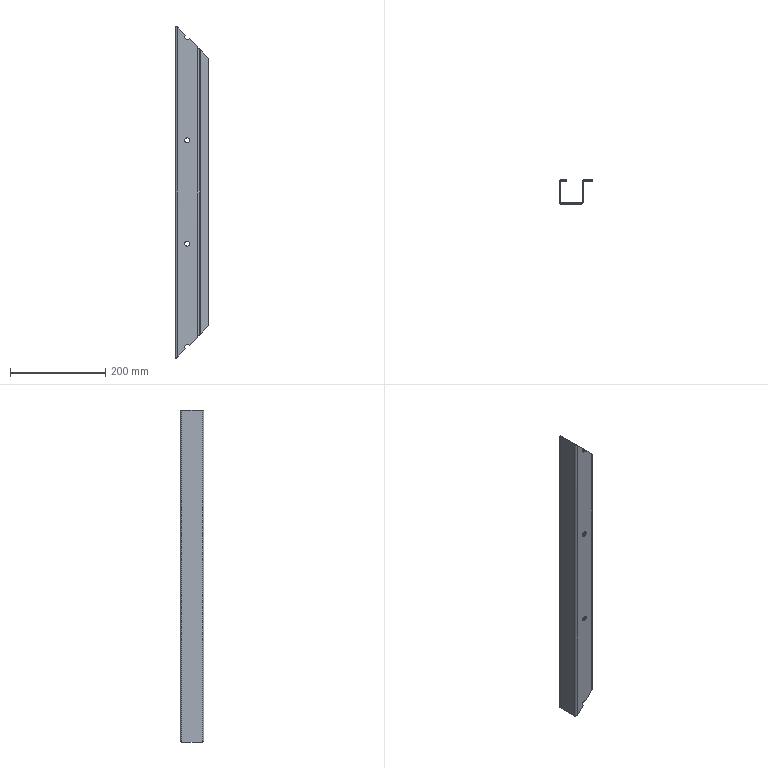Part | STEP file | 750038470 | 1 solid | 47 faces | box 70 x 50 x 696 mm | volume 223150 mm3 | plane 24 | cylinder 15 | spline 8 | commonest cylinder face diameters 10.5 x7 4 x4 8 x4